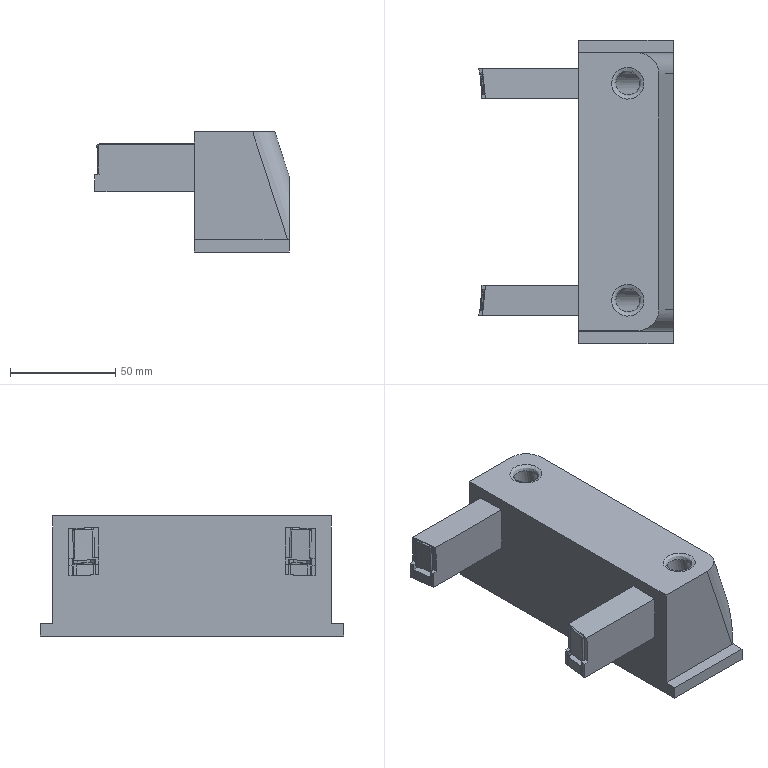Part | NX | features solid 2 | 1 solid | 126 faces | box 92.291 x 144 x 57 mm | volume 348793 mm3 | spline 83 | plane 35 | cylinder 8 | commonest cylinder face diameters 2 x4 11 x2 20 x2